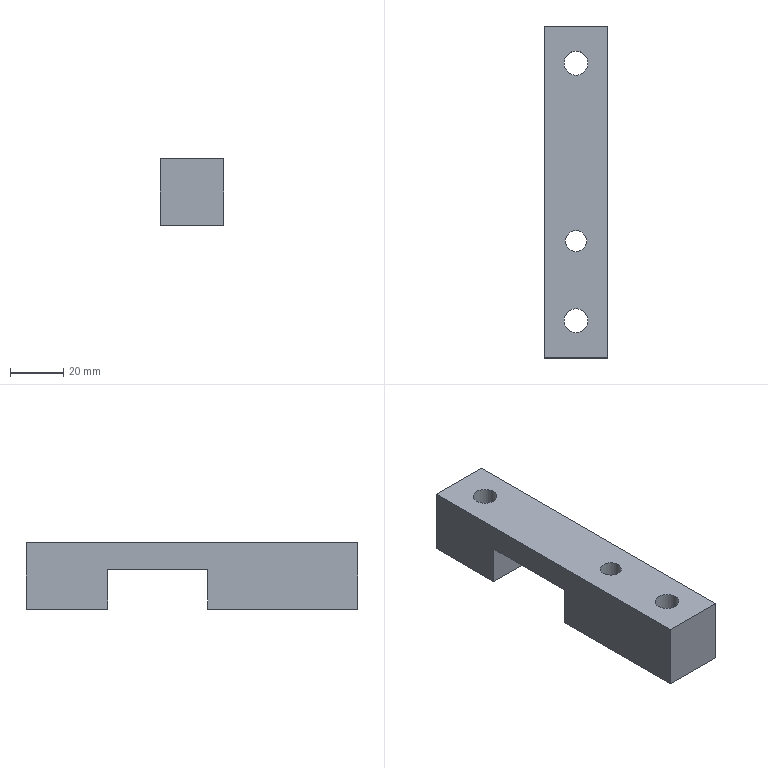Part | STEP file | lll_id2742_x_t | 1 solid | 17 faces | box 24 x 125 x 25 mm | volume 54377 mm3 | plane 12 | cylinder 5 | commonest cylinder face diameters 9 x2 14 x2 8 x1
STEP:
#1=CARTESIAN_POINT('',(3132.435,186.,0.));
#2=VERTEX_POINT('',#1);
#3=CARTESIAN_POINT('',(3139.435,186.,0.));
#4=DIRECTION('',(0.,0.,1.));
#5=DIRECTION('',(-1.,0.,0.));
#6=AXIS2_PLACEMENT_3D('',#3,#4,#5);
#7=CIRCLE('',#6,7.);
#8=EDGE_CURVE('',#2,#2,#7,.T.);
#9=ORIENTED_EDGE('',*,*,#8,.T.);
#10=EDGE_LOOP('',(#9));
#11=FACE_BOUND('',#10,.T.);
#12=CARTESIAN_POINT('',(3127.435,169.221,0.));
#13=VERTEX_POINT('',#12);
#14=CARTESIAN_POINT('',(3127.435,200.,0.));
#15=VERTEX_POINT('',#14);
#16=CARTESIAN_POINT('',(3127.435,4.,0.));
#17=DIRECTION('',(0.,1.,0.));
#18=VECTOR('',#17,1.);
#19=LINE('',#16,#18);
#20=EDGE_CURVE('',#13,#15,#19,.T.);
#21=ORIENTED_EDGE('',*,*,#20,.T.);
#22=CARTESIAN_POINT('',(3151.435,200.,0.));
#23=VERTEX_POINT('',#22);
#24=CARTESIAN_POINT('',(3139.435,200.,0.));
#25=DIRECTION('',(-1.,0.,0.));
#26=VECTOR('',#25,1.);
#27=LINE('',#24,#26);
#28=EDGE_CURVE('',#23,#15,#27,.T.);
#29=ORIENTED_EDGE('',*,*,#28,.F.);
#30=CARTESIAN_POINT('',(3151.435,169.221,0.));
#31=VERTEX_POINT('',#30);
#32=CARTESIAN_POINT('',(3151.435,4.,0.));
#33=DIRECTION('',(0.,1.,0.));
#34=VECTOR('',#33,1.);
#35=LINE('',#32,#34);
#36=EDGE_CURVE('',#31,#23,#35,.T.);
#37=ORIENTED_EDGE('',*,*,#36,.F.);
#38=CARTESIAN_POINT('',(3134.141,169.221,0.));
#39=DIRECTION('',(1.,0.,0.));
#40=VECTOR('',#39,1.);
#41=LINE('',#38,#40);
#42=EDGE_CURVE('',#13,#31,#41,.T.);
#43=ORIENTED_EDGE('',*,*,#42,.F.);
#44=EDGE_LOOP('',(#21,#29,#37,#43));
#45=FACE_BOUND('',#44,.T.);
#46=CARTESIAN_POINT('',(3164.435,-176.117,0.));
#47=DIRECTION('',(0.,0.,-1.));
#48=DIRECTION('',(-1.,0.,0.));
#49=AXIS2_PLACEMENT_3D('',#46,#47,#48);
#50=PLANE('',#49);
#51=ADVANCED_FACE('',(#11,#45),#50,.T.);
#52=CARTESIAN_POINT('',(3135.435,119.,0.));
#53=VERTEX_POINT('',#52);
#54=CARTESIAN_POINT('',(3139.435,119.,0.));
#55=DIRECTION('',(0.,0.,-1.));
#56=DIRECTION('',(-1.,0.,0.));
#57=AXIS2_PLACEMENT_3D('',#54,#55,#56);
#58=CIRCLE('',#57,4.);
#59=EDGE_CURVE('',#53,#53,#58,.T.);
#60=ORIENTED_EDGE('',*,*,#59,.F.);
#61=EDGE_LOOP('',(#60));
#62=FACE_BOUND('',#61,.T.);
#63=CARTESIAN_POINT('',(3132.435,89.,0.));
#64=VERTEX_POINT('',#63);
#65=CARTESIAN_POINT('',(3139.435,89.,0.));
#66=DIRECTION('',(0.,0.,1.));
#67=DIRECTION('',(-1.,0.,0.));
#68=AXIS2_PLACEMENT_3D('',#65,#66,#67);
#69=CIRCLE('',#68,7.);
#70=EDGE_CURVE('',#64,#64,#69,.T.);
#71=ORIENTED_EDGE('',*,*,#70,.T.);
#72=EDGE_LOOP('',(#71));
#73=FACE_BOUND('',#72,.T.);
#74=CARTESIAN_POINT('',(3151.435,75.,0.));
#75=VERTEX_POINT('',#74);
#76=CARTESIAN_POINT('',(3151.435,131.536,0.));
#77=VERTEX_POINT('',#76);
#78=CARTESIAN_POINT('',(3151.435,4.,0.));
#79=DIRECTION('',(0.,1.,0.));
#80=VECTOR('',#79,1.);
#81=LINE('',#78,#80);
#82=EDGE_CURVE('',#75,#77,#81,.T.);
#83=ORIENTED_EDGE('',*,*,#82,.F.);
#84=CARTESIAN_POINT('',(3127.435,75.,0.));
#85=VERTEX_POINT('',#84);
#86=CARTESIAN_POINT('',(3164.435,75.,0.));
#87=DIRECTION('',(1.,0.,0.));
#88=VECTOR('',#87,1.);
#89=LINE('',#86,#88);
#90=EDGE_CURVE('',#85,#75,#89,.T.);
#91=ORIENTED_EDGE('',*,*,#90,.F.);
#92=CARTESIAN_POINT('',(3127.435,131.536,0.));
#93=VERTEX_POINT('',#92);
#94=CARTESIAN_POINT('',(3127.435,4.,0.));
#95=DIRECTION('',(0.,1.,0.));
#96=VECTOR('',#95,1.);
#97=LINE('',#94,#96);
#98=EDGE_CURVE('',#85,#93,#97,.T.);
#99=ORIENTED_EDGE('',*,*,#98,.T.);
#100=CARTESIAN_POINT('',(3134.141,131.536,0.));
#101=DIRECTION('',(-1.,0.,0.));
#102=VECTOR('',#101,1.);
#103=LINE('',#100,#102);
#104=EDGE_CURVE('',#77,#93,#103,.T.);
#105=ORIENTED_EDGE('',*,*,#104,.F.);
#106=EDGE_LOOP('',(#83,#91,#99,#105));
#107=FACE_BOUND('',#106,.T.);
#108=CARTESIAN_POINT('',(3164.435,-176.117,0.));
#109=DIRECTION('',(0.,0.,-1.));
#110=DIRECTION('',(-1.,0.,0.));
#111=AXIS2_PLACEMENT_3D('',#108,#109,#110);
#112=PLANE('',#111);
#113=ADVANCED_FACE('',(#62,#73,#107),#112,.T.);
#114=CARTESIAN_POINT('',(3146.435,89.,14.5));
#115=VERTEX_POINT('',#114);
#116=CARTESIAN_POINT('',(3139.435,89.,14.5));
#117=DIRECTION('',(0.,0.,-1.));
#118=DIRECTION('',(1.,0.,0.));
#119=AXIS2_PLACEMENT_3D('',#116,#117,#118);
#120=CIRCLE('',#119,7.);
#121=EDGE_CURVE('',#115,#115,#120,.T.);
#122=ORIENTED_EDGE('',*,*,#121,.F.);
#123=EDGE_LOOP('',(#122));
#124=FACE_BOUND('',#123,.T.);
#125=ORIENTED_EDGE('',*,*,#70,.F.);
#126=EDGE_LOOP('',(#125));
#127=FACE_BOUND('',#126,.T.);
#128=CARTESIAN_POINT('',(3139.435,89.,2.5));
#129=DIRECTION('',(0.,0.,1.));
#130=DIRECTION('',(1.,0.,0.));
#131=AXIS2_PLACEMENT_3D('',#128,#129,#130);
#132=CYLINDRICAL_SURFACE('',#131,7.);
#133=ADVANCED_FACE('',(#124,#127),#132,.F.);
#134=CARTESIAN_POINT('',(3146.435,186.,14.5));
#135=VERTEX_POINT('',#134);
#136=CARTESIAN_POINT('',(3139.435,186.,14.5));
#137=DIRECTION('',(0.,0.,-1.));
#138=DIRECTION('',(1.,0.,0.));
#139=AXIS2_PLACEMENT_3D('',#136,#137,#138);
#140=CIRCLE('',#139,7.);
#141=EDGE_CURVE('',#135,#135,#140,.T.);
#142=ORIENTED_EDGE('',*,*,#141,.F.);
#143=EDGE_LOOP('',(#142));
#144=FACE_BOUND('',#143,.T.);
#145=ORIENTED_EDGE('',*,*,#8,.F.);
#146=EDGE_LOOP('',(#145));
#147=FACE_BOUND('',#146,.T.);
#148=CARTESIAN_POINT('',(3139.435,186.,2.5));
#149=DIRECTION('',(0.,0.,1.));
#150=DIRECTION('',(1.,0.,0.));
#151=AXIS2_PLACEMENT_3D('',#148,#149,#150);
#152=CYLINDRICAL_SURFACE('',#151,7.);
#153=ADVANCED_FACE('',(#144,#147),#152,.F.);
#154=CARTESIAN_POINT('',(3151.435,131.536,15.));
#155=VERTEX_POINT('',#154);
#156=CARTESIAN_POINT('',(3151.435,169.221,15.));
#157=VERTEX_POINT('',#156);
#158=CARTESIAN_POINT('',(3151.435,4.,15.));
#159=DIRECTION('',(0.,1.,0.));
#160=VECTOR('',#159,1.);
#161=LINE('',#158,#160);
#162=EDGE_CURVE('',#155,#157,#161,.T.);
#163=ORIENTED_EDGE('',*,*,#162,.T.);
#164=CARTESIAN_POINT('',(3151.435,169.221,2.5));
#165=DIRECTION('',(0.,0.,-1.));
#166=VECTOR('',#165,1.);
#167=LINE('',#164,#166);
#168=EDGE_CURVE('',#157,#31,#167,.T.);
#169=ORIENTED_EDGE('',*,*,#168,.T.);
#170=ORIENTED_EDGE('',*,*,#36,.T.);
#171=CARTESIAN_POINT('',(3151.435,200.,25.));
#172=VERTEX_POINT('',#171);
#173=CARTESIAN_POINT('',(3151.435,200.,-652.5));
#174=DIRECTION('',(0.,0.,-1.));
#175=VECTOR('',#174,1.);
#176=LINE('',#173,#175);
#177=EDGE_CURVE('',#172,#23,#176,.T.);
#178=ORIENTED_EDGE('',*,*,#177,.F.);
#179=CARTESIAN_POINT('',(3151.435,75.,25.));
#180=VERTEX_POINT('',#179);
#181=CARTESIAN_POINT('',(3151.435,4.,25.));
#182=DIRECTION('',(0.,-1.,0.));
#183=VECTOR('',#182,1.);
#184=LINE('',#181,#183);
#185=EDGE_CURVE('',#172,#180,#184,.T.);
#186=ORIENTED_EDGE('',*,*,#185,.T.);
#187=CARTESIAN_POINT('',(3151.435,75.,40.));
#188=DIRECTION('',(0.,0.,-1.));
#189=VECTOR('',#188,1.);
#190=LINE('',#187,#189);
#191=EDGE_CURVE('',#180,#75,#190,.T.);
#192=ORIENTED_EDGE('',*,*,#191,.T.);
#193=ORIENTED_EDGE('',*,*,#82,.T.);
#194=CARTESIAN_POINT('',(3151.435,131.536,2.5));
#195=DIRECTION('',(0.,0.,-1.));
#196=VECTOR('',#195,1.);
#197=LINE('',#194,#196);
#198=EDGE_CURVE('',#155,#77,#197,.T.);
#199=ORIENTED_EDGE('',*,*,#198,.F.);
#200=EDGE_LOOP('',(#163,#169,#170,#178,#186,#192,#193,#199));
#201=FACE_OUTER_BOUND('',#200,.T.);
#202=CARTESIAN_POINT('',(3151.435,4.,-652.5));
#203=DIRECTION('',(-1.,0.,0.));
#204=DIRECTION('',(0.,0.,1.));
#205=AXIS2_PLACEMENT_3D('',#202,#203,#204);
#206=PLANE('',#205);
#207=ADVANCED_FACE('',(#201),#206,.F.);
#208=CARTESIAN_POINT('',(3143.935,186.,25.));
#209=VERTEX_POINT('',#208);
#210=CARTESIAN_POINT('',(3139.435,186.,25.));
#211=DIRECTION('',(0.,0.,-1.));
#212=DIRECTION('',(1.,0.,0.));
#213=AXIS2_PLACEMENT_3D('',#210,#211,#212);
#214=CIRCLE('',#213,4.5);
#215=EDGE_CURVE('',#209,#209,#214,.T.);
#216=ORIENTED_EDGE('',*,*,#215,.T.);
#217=EDGE_LOOP('',(#216));
#218=FACE_BOUND('',#217,.T.);
#219=CARTESIAN_POINT('',(3143.935,89.,25.));
#220=VERTEX_POINT('',#219);
#221=CARTESIAN_POINT('',(3139.435,89.,25.));
#222=DIRECTION('',(0.,0.,-1.));
#223=DIRECTION('',(1.,0.,0.));
#224=AXIS2_PLACEMENT_3D('',#221,#222,#223);
#225=CIRCLE('',#224,4.5);
#226=EDGE_CURVE('',#220,#220,#225,.T.);
#227=ORIENTED_EDGE('',*,*,#226,.T.);
#228=EDGE_LOOP('',(#227));
#229=FACE_BOUND('',#228,.T.);
#230=CARTESIAN_POINT('',(3143.435,119.,25.));
#231=VERTEX_POINT('',#230);
#232=CARTESIAN_POINT('',(3139.435,119.,25.));
#233=DIRECTION('',(0.,0.,-1.));
#234=DIRECTION('',(1.,0.,0.));
#235=AXIS2_PLACEMENT_3D('',#232,#233,#234);
#236=CIRCLE('',#235,4.);
#237=EDGE_CURVE('',#231,#231,#236,.T.);
#238=ORIENTED_EDGE('',*,*,#237,.T.);
#239=EDGE_LOOP('',(#238));
#240=FACE_BOUND('',#239,.T.);
#241=CARTESIAN_POINT('',(3127.435,200.,25.));
#242=VERTEX_POINT('',#241);
#243=CARTESIAN_POINT('',(3164.435,200.,25.));
#244=DIRECTION('',(-1.,0.,0.));
#245=VECTOR('',#244,1.);
#246=LINE('',#243,#245);
#247=EDGE_CURVE('',#172,#242,#246,.T.);
#248=ORIENTED_EDGE('',*,*,#247,.T.);
#249=CARTESIAN_POINT('',(3127.435,75.,25.));
#250=VERTEX_POINT('',#249);
#251=CARTESIAN_POINT('',(3127.435,4.,25.));
#252=DIRECTION('',(0.,-1.,0.));
#253=VECTOR('',#252,1.);
#254=LINE('',#251,#253);
#255=EDGE_CURVE('',#242,#250,#254,.T.);
#256=ORIENTED_EDGE('',*,*,#255,.T.);
#257=CARTESIAN_POINT('',(3164.435,75.,25.));
#258=DIRECTION('',(1.,0.,0.));
#259=VECTOR('',#258,1.);
#260=LINE('',#257,#259);
#261=EDGE_CURVE('',#250,#180,#260,.T.);
#262=ORIENTED_EDGE('',*,*,#261,.T.);
#263=ORIENTED_EDGE('',*,*,#185,.F.);
#264=EDGE_LOOP('',(#248,#256,#262,#263));
#265=FACE_BOUND('',#264,.T.);
#266=CARTESIAN_POINT('',(3164.435,236.117,25.));
#267=DIRECTION('',(0.,0.,1.));
#268=DIRECTION('',(1.,0.,0.));
#269=AXIS2_PLACEMENT_3D('',#266,#267,#268);
#270=PLANE('',#269);
#271=ADVANCED_FACE('',(#218,#229,#240,#265),#270,.T.);
#272=CARTESIAN_POINT('',(3127.435,169.221,15.));
#273=VERTEX_POINT('',#272);
#274=CARTESIAN_POINT('',(3127.435,169.221,-652.5));
#275=DIRECTION('',(0.,0.,1.));
#276=VECTOR('',#275,1.);
#277=LINE('',#274,#276);
#278=EDGE_CURVE('',#13,#273,#277,.T.);
#279=ORIENTED_EDGE('',*,*,#278,.T.);
#280=CARTESIAN_POINT('',(3127.435,131.536,15.));
#281=VERTEX_POINT('',#280);
#282=CARTESIAN_POINT('',(3127.435,13712.786,15.));
#283=DIRECTION('',(0.,-1.,0.));
#284=VECTOR('',#283,1.);
#285=LINE('',#282,#284);
#286=EDGE_CURVE('',#273,#281,#285,.T.);
#287=ORIENTED_EDGE('',*,*,#286,.T.);
#288=CARTESIAN_POINT('',(3127.435,131.536,-652.5));
#289=DIRECTION('',(0.,0.,-1.));
#290=VECTOR('',#289,1.);
#291=LINE('',#288,#290);
#292=EDGE_CURVE('',#281,#93,#291,.T.);
#293=ORIENTED_EDGE('',*,*,#292,.T.);
#294=ORIENTED_EDGE('',*,*,#98,.F.);
#295=CARTESIAN_POINT('',(3127.435,75.,-652.5));
#296=DIRECTION('',(0.,0.,1.));
#297=VECTOR('',#296,1.);
#298=LINE('',#295,#297);
#299=EDGE_CURVE('',#85,#250,#298,.T.);
#300=ORIENTED_EDGE('',*,*,#299,.T.);
#301=ORIENTED_EDGE('',*,*,#255,.F.);
#302=CARTESIAN_POINT('',(3127.435,200.,40.));
#303=DIRECTION('',(0.,0.,1.));
#304=VECTOR('',#303,1.);
#305=LINE('',#302,#304);
#306=EDGE_CURVE('',#15,#242,#305,.T.);
#307=ORIENTED_EDGE('',*,*,#306,.F.);
#308=ORIENTED_EDGE('',*,*,#20,.F.);
#309=EDGE_LOOP('',(#279,#287,#293,#294,#300,#301,#307,#308));
#310=FACE_OUTER_BOUND('',#309,.T.);
#311=CARTESIAN_POINT('',(3127.435,4.,-652.5));
#312=DIRECTION('',(-1.,0.,0.));
#313=DIRECTION('',(0.,0.,1.));
#314=AXIS2_PLACEMENT_3D('',#311,#312,#313);
#315=PLANE('',#314);
#316=ADVANCED_FACE('',(#310),#315,.T.);
#317=ORIENTED_EDGE('',*,*,#90,.T.);
#318=ORIENTED_EDGE('',*,*,#191,.F.);
#319=ORIENTED_EDGE('',*,*,#261,.F.);
#320=ORIENTED_EDGE('',*,*,#299,.F.);
#321=EDGE_LOOP('',(#317,#318,#319,#320));
#322=FACE_OUTER_BOUND('',#321,.T.);
#323=CARTESIAN_POINT('',(3425.435,75.,40.));
#324=DIRECTION('',(0.,1.,0.));
#325=DIRECTION('',(0.,0.,-1.));
#326=AXIS2_PLACEMENT_3D('',#323,#324,#325);
#327=PLANE('',#326);
#328=ADVANCED_FACE('',(#322),#327,.F.);
#329=ORIENTED_EDGE('',*,*,#247,.F.);
#330=ORIENTED_EDGE('',*,*,#177,.T.);
#331=ORIENTED_EDGE('',*,*,#28,.T.);
#332=ORIENTED_EDGE('',*,*,#306,.T.);
#333=EDGE_LOOP('',(#329,#330,#331,#332));
#334=FACE_OUTER_BOUND('',#333,.T.);
#335=CARTESIAN_POINT('',(3139.435,200.,40.));
#336=DIRECTION('',(0.,-1.,0.));
#337=DIRECTION('',(0.,0.,1.));
#338=AXIS2_PLACEMENT_3D('',#335,#336,#337);
#339=PLANE('',#338);
#340=ADVANCED_FACE('',(#334),#339,.F.);
#341=CARTESIAN_POINT('',(14054.318,131.536,15.));
#342=DIRECTION('',(1.,0.,0.));
#343=VECTOR('',#342,1.);
#344=LINE('',#341,#343);
#345=EDGE_CURVE('',#281,#155,#344,.T.);
#346=ORIENTED_EDGE('',*,*,#345,.F.);
#347=ORIENTED_EDGE('',*,*,#286,.F.);
#348=CARTESIAN_POINT('',(14054.318,169.221,15.));
#349=DIRECTION('',(-1.,0.,0.));
#350=VECTOR('',#349,1.);
#351=LINE('',#348,#350);
#352=EDGE_CURVE('',#157,#273,#351,.T.);
#353=ORIENTED_EDGE('',*,*,#352,.F.);
#354=ORIENTED_EDGE('',*,*,#162,.F.);
#355=EDGE_LOOP('',(#346,#347,#353,#354));
#356=FACE_OUTER_BOUND('',#355,.T.);
#357=CARTESIAN_POINT('',(14054.318,13712.786,15.));
#358=DIRECTION('',(0.,0.,-1.));
#359=DIRECTION('',(-1.,0.,0.));
#360=AXIS2_PLACEMENT_3D('',#357,#358,#359);
#361=PLANE('',#360);
#362=ADVANCED_FACE('',(#356),#361,.T.);
#363=ORIENTED_EDGE('',*,*,#237,.F.);
#364=EDGE_LOOP('',(#363));
#365=FACE_BOUND('',#364,.T.);
#366=ORIENTED_EDGE('',*,*,#59,.T.);
#367=EDGE_LOOP('',(#366));
#368=FACE_BOUND('',#367,.T.);
#369=CARTESIAN_POINT('',(3139.435,119.,-2.5));
#370=DIRECTION('',(0.,0.,1.));
#371=DIRECTION('',(1.,0.,0.));
#372=AXIS2_PLACEMENT_3D('',#369,#370,#371);
#373=CYLINDRICAL_SURFACE('',#372,4.);
#374=ADVANCED_FACE('',(#365,#368),#373,.F.);
#375=ORIENTED_EDGE('',*,*,#226,.F.);
#376=EDGE_LOOP('',(#375));
#377=FACE_BOUND('',#376,.T.);
#378=CARTESIAN_POINT('',(3143.935,89.,14.5));
#379=VERTEX_POINT('',#378);
#380=CARTESIAN_POINT('',(3139.435,89.,14.5));
#381=DIRECTION('',(0.,0.,-1.));
#382=DIRECTION('',(1.,0.,0.));
#383=AXIS2_PLACEMENT_3D('',#380,#381,#382);
#384=CIRCLE('',#383,4.5);
#385=EDGE_CURVE('',#379,#379,#384,.T.);
#386=ORIENTED_EDGE('',*,*,#385,.T.);
#387=EDGE_LOOP('',(#386));
#388=FACE_BOUND('',#387,.T.);
#389=CARTESIAN_POINT('',(3139.435,89.,-40.5));
#390=DIRECTION('',(0.,0.,1.));
#391=DIRECTION('',(1.,0.,0.));
#392=AXIS2_PLACEMENT_3D('',#389,#390,#391);
#393=CYLINDRICAL_SURFACE('',#392,4.5);
#394=ADVANCED_FACE('',(#377,#388),#393,.F.);
#395=ORIENTED_EDGE('',*,*,#385,.F.);
#396=EDGE_LOOP('',(#395));
#397=FACE_BOUND('',#396,.T.);
#398=ORIENTED_EDGE('',*,*,#121,.T.);
#399=EDGE_LOOP('',(#398));
#400=FACE_BOUND('',#399,.T.);
#401=CARTESIAN_POINT('',(3139.435,89.,14.5));
#402=DIRECTION('',(0.,0.,1.));
#403=DIRECTION('',(1.,0.,0.));
#404=AXIS2_PLACEMENT_3D('',#401,#402,#403);
#405=PLANE('',#404);
#406=ADVANCED_FACE('',(#397,#400),#405,.F.);
#407=ORIENTED_EDGE('',*,*,#215,.F.);
#408=EDGE_LOOP('',(#407));
#409=FACE_BOUND('',#408,.T.);
#410=CARTESIAN_POINT('',(3143.935,186.,14.5));
#411=VERTEX_POINT('',#410);
#412=CARTESIAN_POINT('',(3139.435,186.,14.5));
#413=DIRECTION('',(0.,0.,-1.));
#414=DIRECTION('',(1.,0.,0.));
#415=AXIS2_PLACEMENT_3D('',#412,#413,#414);
#416=CIRCLE('',#415,4.5);
#417=EDGE_CURVE('',#411,#411,#416,.T.);
#418=ORIENTED_EDGE('',*,*,#417,.T.);
#419=EDGE_LOOP('',(#418));
#420=FACE_BOUND('',#419,.T.);
#421=CARTESIAN_POINT('',(3139.435,186.,-40.5));
#422=DIRECTION('',(0.,0.,1.));
#423=DIRECTION('',(1.,0.,0.));
#424=AXIS2_PLACEMENT_3D('',#421,#422,#423);
#425=CYLINDRICAL_SURFACE('',#424,4.5);
#426=ADVANCED_FACE('',(#409,#420),#425,.F.);
#427=ORIENTED_EDGE('',*,*,#417,.F.);
#428=EDGE_LOOP('',(#427));
#429=FACE_BOUND('',#428,.T.);
#430=ORIENTED_EDGE('',*,*,#141,.T.);
#431=EDGE_LOOP('',(#430));
#432=FACE_BOUND('',#431,.T.);
#433=CARTESIAN_POINT('',(3139.435,186.,14.5));
#434=DIRECTION('',(0.,0.,1.));
#435=DIRECTION('',(1.,0.,0.));
#436=AXIS2_PLACEMENT_3D('',#433,#434,#435);
#437=PLANE('',#436);
#438=ADVANCED_FACE('',(#429,#432),#437,.F.);
#439=ORIENTED_EDGE('',*,*,#278,.F.);
#440=ORIENTED_EDGE('',*,*,#42,.T.);
#441=ORIENTED_EDGE('',*,*,#168,.F.);
#442=ORIENTED_EDGE('',*,*,#352,.T.);
#443=EDGE_LOOP('',(#439,#440,#441,#442));
#444=FACE_OUTER_BOUND('',#443,.T.);
#445=CARTESIAN_POINT('',(3134.141,169.221,0.));
#446=DIRECTION('',(0.,1.,0.));
#447=DIRECTION('',(0.,0.,-1.));
#448=AXIS2_PLACEMENT_3D('',#445,#446,#447);
#449=PLANE('',#448);
#450=ADVANCED_FACE('',(#444),#449,.F.);
#451=ORIENTED_EDGE('',*,*,#292,.F.);
#452=ORIENTED_EDGE('',*,*,#345,.T.);
#453=ORIENTED_EDGE('',*,*,#198,.T.);
#454=ORIENTED_EDGE('',*,*,#104,.T.);
#455=EDGE_LOOP('',(#451,#452,#453,#454));
#456=FACE_OUTER_BOUND('',#455,.T.);
#457=CARTESIAN_POINT('',(3134.141,131.536,0.));
#458=DIRECTION('',(0.,-1.,0.));
#459=DIRECTION('',(0.,0.,1.));
#460=AXIS2_PLACEMENT_3D('',#457,#458,#459);
#461=PLANE('',#460);
#462=ADVANCED_FACE('',(#456),#461,.F.);
#463=CLOSED_SHELL('',(#51,#113,#133,#153,#207,#271,#316,#328,#340,#362,#374,#394,#406,#426,#438,#450,#462));
#464=MANIFOLD_SOLID_BREP('',#463);
#465=(LENGTH_UNIT()NAMED_UNIT(*)SI_UNIT(.MILLI.,.METRE.));
#466=UNCERTAINTY_MEASURE_WITH_UNIT(LENGTH_MEASURE(0.00002),#465,'','');
#467=(NAMED_UNIT(*)PLANE_ANGLE_UNIT()SI_UNIT($,.RADIAN.));
#468=PLANE_ANGLE_MEASURE_WITH_UNIT(PLANE_ANGLE_MEASURE(0.01745),#467);
#469=DIMENSIONAL_EXPONENTS(0.,0.,0.,0.,0.,0.,0.);
#470=(CONVERSION_BASED_UNIT('DEGREE',#468)NAMED_UNIT(#469)PLANE_ANGLE_UNIT());
#471=(NAMED_UNIT(*)SI_UNIT($,.STERADIAN.)SOLID_ANGLE_UNIT());
#472=(GEOMETRIC_REPRESENTATION_CONTEXT(3)GLOBAL_UNCERTAINTY_ASSIGNED_CONTEXT((#466))GLOBAL_UNIT_ASSIGNED_CONTEXT((#465,#470,#471))REPRESENTATION_CONTEXT('',''));
#473=ADVANCED_BREP_SHAPE_REPRESENTATION('',(#464),#472);